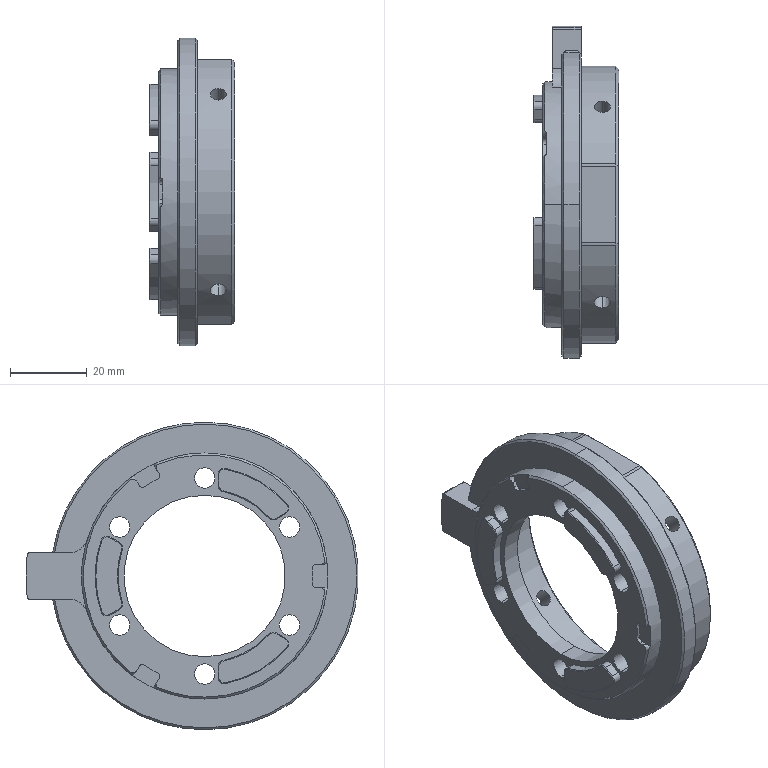NC program | NX | posted with a generic post | part box 22.3 x 86.5 x 80 mm
Lines 26 to 918 of 5076:
(ADAPTIVE_MILLING , TOOL : D10)
N50 T15 M6
N52 G54
N54 G17 G0 G90 X-4.653 Y56.531 S9500 M3
N56 G43 Z30. H15
N58 Z-6.65
N60 G94 G1 Z-9.65 F1000.
N62 X-3.84 Y54.685 F3000.
N64 G3 X-3.278 Y54.149 R1.037
N66 X0.063 Y53.446 R11.74
N68 G2 X10.957 Y51.983 R92.322
N70 X21.093 Y-48.726 R53.11
N72 X10.608 Y-52.015 R70.332
N74 X-18.884 Y49.643 R53.097
N76 X-6.289 Y52.703 R48.18
N78 X0.697 Y52.342 R58.37
N80 X16.022 Y49.494 R65.497
N82 X21.686 Y-47.254 R51.997
N84 X6.969 Y-51.539 R57.357
N86 X-8.626 Y51.279 R52.004
N88 X-0.017 Y51.329 R42.561
N90 X17.335 Y47.887 R62.906
N92 X21.905 Y-45.936 R50.899
N94 X2.392 Y-50.859 R52.826
N96 X-10.178 Y49.875 R50.908
N98 X-0.21 Y50.264 R42.519
N100 X18.185 Y46.397 R60.421
N102 X22.205 Y-44.565 R49.801
N104 X-9.796 Y-48.853 R50.201
N106 X-11.56 Y48.443 R49.811
N108 X0.13 Y49.146 R42.043
N110 X21.213 Y43.868 R55.715
N112 X22.461 Y-43.198 R48.692
N114 X-32.276 Y-36.499 R48.73
N116 X-12.273 Y47.121 R48.677
N118 X0.894 Y48.004 R42.902
N120 X24.046 Y41.104 R52.716
N122 X-47.352 Y5.075 R-47.611
N124 X-12.915 Y45.793 R47.427
N126 X1.477 Y46.867 R43.257
N128 X25.746 Y38.738 R50.676
N130 X7.524 Y-45.874 R46.505
N132 X-14.308 Y44.224 R46.481
N134 X1.271 Y45.786 R42.061
N136 X25.805 Y37.358 R49.355
N138 X-30.481 Y33.648 R-45.391
N140 X-11.505 Y43.805 R43.273
N142 X5.636 Y44.174 R45.023
N144 X31.172 Y31.456 R46.358
N146 X-43.184 Y-9.848 R-44.283
N148 G1 X-43.338 Y-9.304
N150 X-43.35 Y-9.254
N152 X-44.049 Y-5.391
N154 X-44.056 Y-5.34
N156 X-44.379 Y-1.424
N158 X-44.381 Y-1.386
N160 X-44.325 Y2.549
N162 X-44.321 Y2.601
N164 G2 X-43.557 Y8.273 R53.663
N166 X-15.414 Y41.482 R44.351
N168 X1.831 Y43.53 R40.876
N170 X27.351 Y33.407 R46.224
N172 X-28.134 Y-32.742 R-43.172
N174 G1 X-28.675 Y-32.358
N176 X-28.715 Y-32.327
N178 X-31.68 Y-29.753
N180 X-31.717 Y-29.718
N182 X-34.419 Y-26.87
N184 X-34.453 Y-26.831
N186 X-36.868 Y-23.736
N188 X-36.897 Y-23.694
N190 X-39.002 Y-20.38
N192 X-39.028 Y-20.335
N194 X-40.803 Y-16.834
N196 X-40.824 Y-16.787
N198 X-42.253 Y-13.13
N200 X-42.269 Y-13.082
N202 X-43.188 Y-9.834
N204 X-43.35 Y-9.254
N206 X-44.056 Y-5.34
N208 X-44.381 Y-1.386
N210 X-44.321 Y2.601
N212 X-43.878 Y6.553
N214 X-43.069 Y10.395
N216 X-43.056 Y10.444
N218 X-41.88 Y14.19
N220 X-41.862 Y14.238
N222 X-40.329 Y17.852
N224 X-40.307 Y17.899
N226 X-38.433 Y21.348
N228 X-38.406 Y21.392
N230 X-36.207 Y24.645
N232 X-36.177 Y24.686
N234 X-33.674 Y27.711
N236 X-33.64 Y27.749
N238 G2 X-22.244 Y37.008 R56.807
N240 X0.983 Y42.477 R39.115
N242 X27.626 Y31.711 R44.927
N244 X-14.28 Y-39.56 R42.064
N246 G1 X-14.359 Y-39.548
N248 X-15.489 Y-39.287
N250 X-15.55 Y-39.269
N252 G2 X-22.305 Y-36.473 R47.797
N254 X-28.225 Y-32.678 R45.06
N256 G3 X-29.238 Y-32.592 R1.011
N258 G1 X-29.749 Y-32.939 Z-9.619
N260 X-30.243 Y-33.309 Z-9.588
N262 X-30.859 Y-33.762 Z-9.55
N264 X-31.349 Y-34.104
N266 G2 X-32.571 Y-33.843 R1.007
N268 G1 X-35.342 Y-30.459
N270 X-38.093 Y-27.059
N272 G2 X-41.623 Y-21.92 R53.328
N274 X-44.301 Y-16.294 R39.22
N276 X-46.227 Y-10.042 R44.417
N278 X-47.09 Y-5.068 R37.184
N280 G1 X-47.188 Y-3.575
N282 X-47.33 Y0.483
N284 G2 X-46.805 Y6.985 R35.819
N286 X-45.43 Y13.064 R46.25
N288 X-43.008 Y19.138 R42.842
N290 X-39.119 Y25.665 R43.353
N292 X-36.629 Y28.956 R54.71
N294 G1 X-35.319 Y30.552
N296 G2 X-34.345 Y30.897 R1.011
N298 G1 X-34.104 Y30.848
N300 X-32.145 Y30.447 Z-9.65
N302 X-31.506 Y30.327
N304 G3 X-30.819 Y30.552 R1.03
N306 G1 X-27.782 Y33.04
N308 X-27.741 Y33.071
N310 X-24.476 Y35.255
N312 X-24.436 Y35.279
N314 G2 X23.116 Y33.792 R44.536
N316 X-10.193 Y-39.65 R40.949
N318 X-14.28 Y-39.56 R39.491
N320 G3 X-15.024 Y-39.814 R1.026
N322 G1 X-15.356 Y-40.113
N324 X-16.842 Y-41.451 Z-9.55
N326 X-17.082 Y-41.665
N328 X-17.354 Y-41.835
N330 G2 X-18.177 Y-41.81 R1.025
N332 G1 X-23.036 Y-39.422
N334 G2 X-28.56 Y-36.11 R54.922
N336 X-32.749 Y-32.961 R38.545
N338 G1 X-33.565 Y-32.19
N340 X-34.348 Y-31.386
N342 X-35.707 Y-29.91
N344 X-37.027 Y-28.399
N346 G2 X-40.835 Y-23.031 R47.098
N348 X-44.729 Y-14.96 R40.767
N350 X-46.551 Y-8.399 R42.555
N352 X-47.46 Y-0.28 R64.723
N354 X-47.088 Y5.656 R31.632
N356 X-45.028 Y14.131 R47.314
N358 X-39.734 Y24.685 R41.336
N360 X-32.675 Y32.889 R48.607
N362 X-27.382 Y36.895 R35.549
N364 X-22.086 Y40.046 R101.
N366 G1 X-19.387 Y41.536
N368 G2 X-18.189 Y41.36 R1.007
N370 G1 X-17.939 Y41.105
N372 X-16.541 Y39.675 Z-9.65
N374 G3 X-15.49 Y39.286 R1.068
N376 G2 X-12.071 Y39.663 R11.505
N378 X-5.099 Y40.283 R788.852
N380 X5.834 Y39.65 R46.86
N382 X9.041 Y39.268 R10.135
N384 X17.719 Y35.709 R71.914
N386 X32.673 Y-22.721 R39.917
N388 X15.112 Y-36.784 R39.741
N390 G1 X12.628 Y-37.96
N392 X12.582 Y-37.979
N394 X9.041 Y-39.268
N396 X8.979 Y-39.287
N398 G2 X6.186 Y-39.662 R10.36
N400 X-3.18 Y-39.688 R68.393
N402 G1 X-3.554 Y-39.653
N404 X-3.587 Y-39.65
N406 X-10.212
N408 G3 X-11.31 Y-40.752 R1.1
N410 X-10.212 Y-41.85 R1.1
N412 G1 X6.561
N414 G3 X7.659 Y-40.748 R1.1
N416 X6.561 Y-39.65 R1.1
N418 G1 X-3.689
N420 G3 X-4.522 Y-40.098 R1.014
N422 G1 X-4.775 Y-40.478
N424 X-5.879 Y-42.146 Z-9.55
N426 X-6.049 Y-42.401
N428 X-6.26 Y-42.624
N430 G2 X-6.871 Y-42.832 R1.041
N432 G1 X-9.403 Y-42.835
N434 X-11.935 Y-42.819
N436 G2 X-17.906 Y-41.586 R19.072
N438 X-29.335 Y-35.547 R42.918
N440 X-33.433 Y-32.201 R48.256
N442 X-35.907 Y-29.643 R36.08
N444 G1 X-38.152 Y-27.046
N446 G2 X-41.775 Y-21.604 R35.141
N448 X-44.145 Y-16.522 R38.315
N450 X-46.489 Y-8.981 R53.416
N452 G1 X-46.942 Y-7.011
N454 X-47.348 Y-5.031
N456 G2 X-47.605 Y-0.784 R20.073
N458 G1 X-47.506 Y1.296
N460 X-47.392 Y3.376
N462 G2 X-46.479 Y9.113 R37.336
N464 X-42.841 Y19.444 R45.999
N466 X-36.22 Y29.286 R48.06
N468 X-28.961 Y35.853 R44.574
N470 X-22.883 Y39.429 R43.932
N472 X-15.628 Y42.832 R163.757
N474 X-14.306 Y42.333 R1.005
N476 G1 X-14.191 Y42.079
N478 X-13.366 Y40.258 Z-9.65
N480 G3 X-12.446 Y39.65 R1.011
N482 G1 X5.929
N484 G2 X7.849 Y39.548 R15.168
N486 G1 X9.041 Y39.268
N488 X12.692 Y37.933
N490 X16.162 Y36.28
N492 X16.206 Y36.256
N494 X19.505 Y34.282
N496 X19.546 Y34.254
N498 X22.643 Y31.977
N500 X22.683 Y31.945
N502 G2 X32.223 Y21.398 R51.83
N504 X28.494 Y-26.13 R38.687
N506 G1 X27.965 Y-26.806
N508 X27.933 Y-26.843
N510 X25.341 Y-29.589
N512 X25.305 Y-29.624
N514 X22.469 Y-32.117
N516 X22.43 Y-32.148
N518 X19.375 Y-34.368
N520 X19.333 Y-34.395
N522 X16.085 Y-36.321
N524 X16.041 Y-36.344
N526 X15.025 Y-36.825
N528 G3 X15.474 Y-38.729 R1.
N530 G1 X16.462 Y-38.579 Z-9.6
N532 X17.448 Y-38.411 Z-9.55
N534 X18.278 Y-38.277
N536 X19.105 Y-38.123
N538 X19.371 Y-37.99
N540 X22.769 Y-35.585
N542 G3 X29.728 Y-29.349 R46.818
N544 G1 X30.412 Y-28.566
N546 X31.083 Y-27.772
N548 X33.246 Y-25.105
N550 G3 X36.758 Y-19.588 R37.102
N552 X38.514 Y-15.936 R42.392
N554 X41.433 Y-4.041 R44.192
N556 G1 X41.547 Y-2.549
N558 X41.615 Y-1.054
N560 X41.661 Y0.773
N562 X41.654 Y2.601
N564 G3 X41.07 Y7.638 R32.422
N566 X39.399 Y13.635 R35.228
N568 X35.669 Y21.665 R55.912
N570 X34.01 Y24.156 R27.546
N572 G1 X30.171 Y29.258
N574 X29.988 Y29.44
N576 X29.768 Y29.575
N578 X28.156 Y30.271
N580 X26.678 Y30.9 Z-9.63
N582 X26.484 Y30.931 Z-9.64
N584 X26.288 Z-9.65
N586 G3 X25.671 Y29.258 R1.002
N588 G1 X28.199 Y26.53
N590 X28.232 Y26.492
N592 X30.566 Y23.438
N594 X30.595 Y23.397
N596 X32.631 Y20.136
N598 X32.655 Y20.092
N600 X34.374 Y16.653
N602 X34.394 Y16.607
N604 X35.779 Y13.022
N606 X35.795 Y12.974
N608 X36.835 Y9.273
N610 X36.847 Y9.224
N612 X37.533 Y5.442
N614 X37.539 Y5.392
N616 X37.865 Y1.559
N618 X37.866 Y1.518
N620 X37.828 Y-2.333
N622 X37.825 Y-2.383
N624 X37.423 Y-6.206
N626 X37.416 Y-6.255
N628 X36.671 Y-9.958
N630 X36.659 Y-10.005
N632 X35.574 Y-13.623
N634 X35.557 Y-13.669
N636 X34.141 Y-17.17
N638 X34.12 Y-17.215
N640 X32.384 Y-20.569
N642 X32.36 Y-20.612
N644 X30.32 Y-23.79
N646 X30.291 Y-23.83
N648 X28.443 Y-26.194
N650 G3 X28.462 Y-27.461 R1.017
N652 G1 X29.548 Y-28.771
N654 Z-6.65
N656 G0 Z30.
N658 X0.053 Y2.944
N660 Z3.
N662 G3 X0.053 Y2.944 Z2.506 I-3.312 J-3.046 F1000.
N664 X0.053 Y2.944 Z2.013 I-3.312 J-3.046
N666 X0.053 Y2.944 Z1.519 I-3.312 J-3.046
N668 X0.053 Y2.944 Z1.026 I-3.312 J-3.046
N670 X0.053 Y2.944 Z0.532 I-3.312 J-3.046
N672 X0.053 Y2.944 Z0.039 I-3.312 J-3.046
N674 X0.053 Y2.944 Z-0.455 I-3.312 J-3.046
N676 X0.053 Y2.944 Z-0.948 I-3.312 J-3.046
N678 X0.053 Y2.944 Z-1.442 I-3.312 J-3.046
N680 X0.053 Y2.944 Z-1.935 I-3.312 J-3.046
N682 X0.053 Y2.944 Z-2.429 I-3.312 J-3.046
N684 X0.053 Y2.944 Z-2.922 I-3.312 J-3.046
N686 X0.053 Y2.944 Z-3.416 I-3.312 J-3.046
N688 X0.053 Y2.944 Z-3.909 I-3.312 J-3.046
N690 X0.053 Y2.944 Z-4.403 I-3.312 J-3.046
N692 X0.053 Y2.944 Z-4.896 I-3.312 J-3.046
N694 X0.053 Y2.944 Z-5.39 I-3.312 J-3.046
N696 X0.053 Y2.944 Z-5.884 I-3.312 J-3.046
N698 X0.053 Y2.944 Z-6.377 I-3.312 J-3.046
N700 X0.053 Y2.944 Z-6.871 I-3.312 J-3.046
N702 X0.053 Y2.944 Z-7.364 I-3.312 J-3.046
N704 X0.053 Y2.944 Z-7.858 I-3.312 J-3.046
N706 X0.053 Y2.944 Z-8.351 I-3.312 J-3.046
N708 X0.053 Y2.944 Z-8.845 I-3.312 J-3.046
N710 X0.053 Y2.944 Z-9.338 I-3.312 J-3.046
N712 X-3.259 Y-4.603 Z-9.65 R-4.5
N714 X-5.865 Y-3.781 R-4.501 F3000.
N716 X1.609 Y0.889 R4.669
N718 X-6.732 Y-3.688 R-4.977
N720 X1.835 Y1.86 R5.197
N722 X-7.337 Y-3.783 R-5.474
N724 X2.339 Y1.985 R5.712
N726 X-8.13 Y-3.624 R-5.991
N728 X2.709 Y2.514 R6.254
N730 X-8.698 Y-3.77 R-6.536
N732 X3.191 Y2.798 R6.809
N734 X-9.24 Y-3.976 R-7.097
N736 X3.814 Y2.819 R7.382
N738 X-9.954 Y-3.925 R-7.68
N740 X4.254 Y3.298 R7.975
N742 X-6.709 Y7.397 R8.276
N744 X-10.803 Y-3.578 R8.276
N746 X4.988 Y3.144 R8.583
N748 X-11.438 Y-3.683 R-8.895
N750 X5.93 Y2.261 R9.205
N752 X-12.334 Y-3.108 R-9.523
N754 X6.323 Y3.189 R-9.846
N756 X-13.025 Y-3.071 R10.17
N758 X7.293 Y2.129 R10.496
N760 X-13.978 Y-1.859 R10.824
N762 X7.973 Y2.133 R-11.158
N764 X-14.681 Y-1.734 R11.495
N766 X8.777 Y1.413 R11.835
N768 X-15.416 Y-1.373 R12.177
N770 X9.55 Y0.428 R12.521
N772 X-16.176 Y-0.278 R12.868
N774 X10.234 Y-0.81 R13.215
N776 X-16.778 Y1.579 R13.566
N778 X10.695 Y-2.8 R13.919
N780 X-16.152 Y6.155 R14.267
N782 X6.568 Y-11.201 R14.599
N784 X-4.293 Y14.898 R14.9
N786 X-12.264 Y-12.37 R15.156
N788 X10.634 Y7.29 R15.458
N790 X-18.688 Y-3.731 R15.797
N792 X13.17 Y0.666 R16.149
N794 X-19.74 Y1.58 R16.506
N796 X12.171 Y-7.529 R16.856
N798 X-12.082 Y14.761 R17.185
N800 X-4.935 Y-17.612 R17.476
N802 X6.808 Y14.833 R17.768
N804 X-19.741 Y-7.704 R18.095
N806 X15.253 Y2.805 R18.443
N808 X-22.054 Y1.453 R18.8
N810 X9.84 Y-14.327 R19.131
N812 X-2.728 Y19.458 R19.411
N814 X-14.168 Y-16.615 R19.699
N816 X11.651 Y13.715 R20.049
N818 X-23.283 Y-4.298 R20.408
N820 X15.361 Y-9.754 R20.734
N822 X-6.801 Y20.738 R21.013
N824 X-8.398 Y-20.911 R21.301
N826 X7.86 Y18.783 R21.658
N828 X-23.028 Y-9.945 R22.019
N830 X19.281 Y2.209 R22.373
N832 X-24.736 Y7.486 R22.714
N834 X3.68 Y-22.196 R23.001
N836 X4.205 Y22.202 R23.297
N838 X-19.564 Y-17.369 R23.649
N840 X14.413 Y-16.478 R24.034
N842 X13.422 Y17.593 R24.034
N844 X-26.964 Y-6.202 R24.417
N846 X16.734 Y-14.996 R24.734
N848 X-4.465 Y25.019 R24.991
N850 X-6.806 Y-25.334 R25.322
N852 X15.378 Y-17.808 R25.62
N854 X21.372 Y-7.798 R25.452
N856 X22.55 Y1.289 R26.802
N858 X21.446 Y7.608 R28.715
N860 X20.209 Y10.843 R132.37
N862 G1 X18.781 Y13.482
N864 X18.719 Y13.59
N866 X18.656 Y13.698
N868 X18.576 Y13.832
N870 G3 X12.82 Y20.239 R27.567
N872 X5.21 Y24.419 R27.805
N874 X-6.101 Y25.69 R26.945
N876 X-16.522 Y22.182 R26.901
N878 X-21.379 Y18.427 R29.922
N880 X-25.212 Y13.636 R29.9
N882 X-27.807 Y8.076 R29.9
N884 X-29.019 Y2.061 R29.9
N886 G1 X-29.086 Y-0.91
N888 X-29.081 Y-1.012
N890 G3 X-28.115 Y-7.071 R29.9
N892 X-25.748 Y-12.732 R29.9
N894 X-22.113 Y-17.675 R29.9
N896 X-17.416 Y-21.622 R29.919
N898 X-9.338 Y-25.121 R27.839
N900 X-3.243 Y-25.849 R29.463
N902 X5.338 Y-24.376 R27.651
N904 X12.913 Y-20.166 R27.811
N906 X16.998 Y-16.058 R29.766
N908 G1 X18.607 Y-13.789
N910 X18.67 Y-13.688
N912 X20.024 Y-11.234
N914 X20.059 Y-11.165
N916 X20.387 Y-10.452
N918 X20.418 Y-10.377
N920 X21.448 Y-7.604
N922 X21.484 Y-7.484
N924 X22.173 Y-4.631
N926 X22.195 Y-4.507
N928 X22.542 Y-1.593
N930 X22.55 Y-1.467
N932 Y1.467
N934 X22.542 Y1.593
N936 X22.528 Y1.717
N938 X21.528 Y7.304
N940 X21.484 Y7.484
N942 X21.448 Y7.604
N944 X20.417 Y10.381
N946 X20.39 Y10.448
N948 X20.338 Y10.562
N950 X18.781 Y13.482
N952 X18.674 Y13.68
N954 X18.607 Y13.788
N956 X18.534 Y13.89
N958 X16.929 Y16.145
N960 X15.08 Y18.217
N962 X14.996 Y18.302
N964 X12.927 Y20.154
N966 X12.834 Y20.229
N968 X10.57 Y21.838
N970 X10.47 Y21.902
N972 X8.04 Y23.248
N974 X7.933 Y23.3
N976 X5.368 Y24.366
N978 X5.256 Y24.405
N980 X2.587 Y25.178
N982 X2.471 Y25.204
N984 X-0.266 Y25.673
N986 X-0.385 Y25.687
N988 X-0.509 Y25.694
N990 X-3.276 Y25.847
N992 X-6.101 Y25.69
N994 G3 X-6.938 Y24.552 R1.015
N996 G1 X-6.727 Y23.051
N998 Z-6.65
N1000 G0 Z30.
N1002 X-4.681 Y56.558
N1004 Z-11.65
N1006 G1 Z-14.65 F1000.
N1008 X-4.221 Y55.549 F3000.
N1010 X-3.742 Y54.549
N1012 G3 X-3.306 Y54.177 R1.063
N1014 X0.027 Y53.447 R10.851
N1016 G2 X11.656 Y51.83 R87.753
N1018 X19.86 Y-49.24 R53.106
N1020 X9.665 Y-52.196 R71.246
N1022 X-46.174 Y26.253 R53.072
N1024 X-6.458 Y52.701 R52.902
N1026 X-0.095 Y52.414 R48.132
N1028 X13.946 Y50.125 R73.166
N1030 X20.702 Y-47.695 R52.006
N1032 X5.029 Y-51.768 R56.719
N1034 X-8.428 Y51.31 R52.004
N1036 X-0.192 Y51.344 R42.16
N1038 X16.582 Y48.157 R63.918
N1040 X21.161 Y-46.288 R50.907
N1042 X0.071 Y-50.92 R52.509
N1044 X-9.984 Y49.908 R50.906
N1046 X0.236 Y50.23 R42.588
N1048 X19.407 Y45.892 R58.753
N1050 X21.243 Y-45.033 R49.789
N1052 X-11.085 Y-48.575 R50.123
N1054 X-11.126 Y48.535 R49.799
N1056 X0.449 Y49.13 R43.234
N1058 X20.825 Y44.053 R55.907
N1060 X9.833 Y-47.686 R48.707
N1062 X-12.209 Y47.135 R48.689
N1064 X1.459 Y47.966 R43.901
N1066 X22.799 Y41.81 R53.127
N1068 X46.724 Y9.218 R47.692
N1070 G3 X47.077 Y8.662 R3.514
N1072 G2 X48.014 Y6.155 R6.549
N1074 X48.351 Y-2.093 R58.322
N1076 G1 X48.014 Y-6.155
N1078 X48. Y-6.24
N1080 G2 X47.149 Y-8.987 R20.531
N1082 X43.865 Y-18.558 R90.92
N1084 X-36.38 Y-30.727 R47.661
N1086 G1 X-36.621 Y-30.44
N1088 X-36.859 Y-30.15
N1090 X-37.106 Y-29.845
N1092 X-39.374 Y-27.089
N1094 X-39.403 Y-27.051
N1096 X-41.7 Y-23.673
N1098 X-41.725 Y-23.632
N1100 X-43.703 Y-20.059
N1102 X-43.725 Y-20.015
N1104 X-45.368 Y-16.276
N1106 X-45.385 Y-16.231
N1108 X-46.68 Y-12.357
N1110 X-46.693 Y-12.311
N1112 X-47.628 Y-8.335
N1114 X-47.637 Y-8.287
N1116 X-48.204 Y-4.242
N1118 X-48.208 Y-4.194
N1120 X-48.404 Y-0.089
N1122 X-48.225 Y4.014
N1124 X-48.221 Y4.063
N1126 X-47.669 Y8.109
N1128 X-47.661 Y8.157
N1130 X-46.742 Y12.137
N1132 X-46.729 Y12.184
N1134 X-45.45 Y16.062
N1136 X-45.433 Y16.108
N1138 X-43.804 Y19.853
N1140 X-43.783 Y19.897
N1142 X-41.819 Y23.478
N1144 X-41.794 Y23.519
N1146 G2 X-31.315 Y35.877 R58.41
N1148 X-11.29 Y46.179 R45.823
N1150 X4.133 Y46.593 R46.615
N1152 X28.226 Y36.971 R49.601
N1154 X45.246 Y10.885 R47.105
N1156 G3 X46.091 Y9.771 R1.581
N1158 G1 X46.187 Y9.687
N1160 X46.934 Y8.846
N1162 G2 X48.014 Y6.155 R6.351
N1164 G1 X48.352 Y2.049
N1166 X48.351 Y-2.093
N1168 X48. Y-6.24
N1170 X47.697 Y-7.455
N1172 X47.652 Y-7.574
N1174 G2 X46.353 Y-9.832 R40.435
N1176 G3 X44.011 Y-15.489 R79.968
N1178 G2 X33.71 Y-32.046 R50.363
N1180 X-21.517 Y-41.238 R46.63
N1182 G1 X-23.602 Y-40.304
N1184 X-23.646 Y-40.282
N1186 X-27.276 Y-38.228
N1188 X-27.318 Y-38.202
N1190 X-30.671 Y-35.871
N1192 X-30.71 Y-35.842
N1194 X-33.837 Y-33.214
N1196 X-33.872 Y-33.181
N1198 X-36.745 Y-30.279
N1200 X-36.778 Y-30.243
N1202 X-37.175 Y-29.76
N1204 G3 X-38.917 Y-30.639 R1.001
N1206 G1 X-38.699 Y-31.166 Z-14.621
N1208 X-38.454 Y-31.681 Z-14.593
N1210 X-38.094 Y-32.46 Z-14.55
N1212 X-37.344 Y-34.059
N1214 X-37.175 Y-34.26
N1216 X-35.796 Y-35.524
N1218 X-34.383 Y-36.749
N1220 G3 X-27.548 Y-41.473 R58.147
N1222 X-19.897 Y-45.227 R67.301
N1224 X-11.651 Y-48.061 R58.6
N1226 G1 X-8.296 Y-48.922
N1228 G3 X-0.624 Y-49.683 R31.054
N1230 X8.044 Y-48.769 R56.237
N1232 G1 X9.946 Y-48.416
N1234 X11.839 Y-48.016
N1236 G3 X19.967 Y-45.217 R44.748
N1238 X25.485 Y-42.32 R46.569
N1240 X30.203 Y-39.272 R79.669
N1242 X33.745 Y-36.388 R29.88
N1244 G1 X34.33 Y-35.798
N1246 X34.902 Y-35.196
N1248 X36.416 Y-33.534
N1250 X37.898 Y-31.845
N1252 G3 X42.477 Y-25.315 R43.327
N1254 X46.666 Y-17.64 R241.213
N1256 G1 X49.255 Y-12.664
N1258 G3 X49.344 Y-11.986 R1.033
N1260 G1 X48.977 Y-10.333
N1262 X48.839 Y-9.689 Z-14.583
N1264 X48.677 Y-9.052 Z-14.616
N1266 G3 X48.229 Y-8.553 Z-14.65 R1.039
N1268 X47.005 Y-8.767 R1.007
N1270 X44.1 Y-13.08 R13.969
N1272 G2 X39.848 Y-21.851 R118.493
N1274 X-5.722 Y-45.034 R45.642
N1276 G1 X-7.47 Y-44.952
N1278 X-7.52 Y-44.947
N1280 X-11.649 Y-44.362
N1282 X-11.697 Y-44.352
N1284 X-15.754 Y-43.384
N1286 X-15.802 Y-43.37
N1288 X-19.75 Y-42.028
N1290 X-19.796 Y-42.01
N1292 X-21.621 Y-41.192
N1294 G3 X-23.022 Y-41.98 R1.003
N1296 X-22.726 Y-42.847 Z-14.603 R1.147
N1298 G1 X-22.106 Y-43.701 Z-14.55
N1300 X-21.541 Y-44.486
N1302 X-20.96 Y-45.26
N1304 G3 X-20.457 Y-45.538 R1.051
N1306 G1 X-15.673 Y-46.574
N1308 X-10.883 Y-47.576
N1310 X-9.424 Y-47.861
N1312 X-7.962 Y-48.13
N1314 G3 X-2.645 Y-48.483 R29.412
N1316 G1 X1.728 Y-48.355
N1318 G3 X9.151 Y-47.451 R56.509
N1320 X19.263 Y-44.358 R41.96
N1322 X24.782 Y-41.466 R44.858
N1324 X31.657 Y-36.687 R60.043
N1326 X35.461 Y-32.949 R31.966
N1328 X42.678 Y-22.8 R58.296
N1330 G1 X45.053 Y-18.368
N1332 X47.402 Y-13.922
N1334 X47.461 Y-13.685
N1336 X47.702 Y-11.701
N1338 X47.787 Y-11.046 Z-14.583
N1340 X47.848 Y-10.388 Z-14.616
N1342 G3 X47.596 Y-9.772 Z-14.65 R1.039
N1344 X46.187 Y-9.687 R1.005
N1346 X43.48 Y-12.744 R8.296
N1348 X40.002 Y-19.388 R218.961
N1350 G2 X26.545 Y-35.441 R47.236
N1352 X10.133 Y-43.082 R44.95
N1354 G1 X9.206 Y-43.395
N1356 X9.159 Y-43.409
N1358 X5.113 Y-44.367
N1360 X5.065 Y-44.376
N1362 X0.947 Y-44.953
N1364 X0.898 Y-44.957
N1366 X-3.279 Y-45.15
N1368 X-5.789 Y-45.031
N1370 G3 X-6.383 Y-46.867 R1.001
N1372 G1 X-6.013 Y-47.036 Z-14.63
N1374 X-5.63 Y-47.174 Z-14.609
N1376 X-4.519 Y-47.587 Z-14.55
N1378 X-2.875 Y-48.19
N1380 X-2.607 Y-48.213
N1382 X-0.74 Y-48.125
N1384 X1.124 Y-47.983
N1386 G3 X10.299 Y-46.184 R63.114
N1388 X15.675 Y-44.551 R76.492
N1390 X22.862 Y-41.294 R47.031
N1392 X31.334 Y-35.317 R45.135
N1394 X35.179 Y-31.526 R61.541
N1396 X40.1 Y-25.091 R52.378
N1398 G1 X40.772 Y-24.039
N1400 X46.741 Y-14.472
N1402 X46.838 Y-14.257
N1404 X46.889 Y-14.026
N1406 X47.045 Y-12.167
N1408 X47.105 Y-11.515 Z-14.583
N1410 X47.14 Y-10.861 Z-14.616
N1412 G3 X46.856 Y-10.247 Z-14.65 R1.038
N1414 X45.576 Y-10.126 R1.007
N1416 X44.053 Y-11.181 R14.835
N1418 X41.169 Y-15.243 R17.512
N1420 G2 X35.721 Y-24.358 R99.276
N1422 X24.897 Y-35.253 R44.428
N1424 G1 X24.157 Y-35.875
N1426 X24.118 Y-35.905
N1428 X20.699 Y-38.27
N1430 X20.657 Y-38.296
N1432 X17.033 Y-40.334
N1434 X16.989 Y-40.356
N1436 X13.191 Y-42.047
N1438 X13.145 Y-42.065
N1440 X10.066 Y-43.105
N1442 G3 X9.669 Y-44.749 R1.002
N1444 X10.44 Y-45.069 Z-14.607 R1.172
N1446 G1 X11.574 Y-45.223 Z-14.55
N1448 X13.355 Y-45.465
N1450 G3 X13.963 Y-45.355 R1.044
N1452 G1 X16.531 Y-43.975
N1454 X19.092 Y-42.583
N1456 G3 X28.738 Y-36.074 R76.978
N1458 X39.109 Y-24.53 R47.964
N1460 X44.965 Y-15.028 R255.2
N1462 G1 X45.034 Y-14.886
N1464 X45.831 Y-12.88
N1466 X46.077 Y-12.278 Z-14.583
N1468 X46.298 Y-11.666 Z-14.615
N1470 G3 X46.199 Y-10.989 Z-14.65 R1.038
N1472 X44.965 Y-10.528 R1.005
N1474 X41.991 Y-12.711 R6.003
N1476 X38.575 Y-17.938 R45.009
N1478 G1 X37.799 Y-19.222
N1480 X37.539 Y-19.649
N1482 X37.211 Y-20.181
N1484 X37.145 Y-20.287
N1486 X36.744 Y-20.921
N1488 X36.543 Y-21.237
N1490 X36.498 Y-21.306
N1492 X35.342 Y-23.425
N1494 X35.316 Y-23.467
N1496 X32.994 Y-26.915
N1498 X32.965 Y-26.955
N1500 X30.332 Y-30.172
N1502 X30.299 Y-30.209
N1504 X27.377 Y-33.167
N1506 X27.341 Y-33.201
N1508 X24.852 Y-35.291
N1510 G3 X26.425 Y-36.813 R-1.1
N1512 G1 X39.107 Y-20.664
N1514 X40.342 Y-19.091 Z-14.55
N1516 X44.957 Y-13.215
N1518 X45.296 Y-12.789 Z-14.577
N1520 X45.618 Y-12.35 Z-14.605
N1522 G3 X45.694 Y-11.469 Z-14.65 R1.127
N1524 X44.263 Y-10.794 R1.104
N1526 X42.364 Y-11.677 R6.484
N1528 X39.174 Y-15.373 R14.727
N1530 G2 X37.333 Y-19.775 R59.519
N1532 G1 X36.495 Y-21.311
N1534 G3 X38.382 Y-22.439 R1.1
N1536 G1 X38.83 Y-21.751
N1538 X39.923 Y-20.076 Z-14.55
N1540 X44.255 Y-13.435
N1542 X44.82 Y-12.549 Z-14.603
N1544 G3 X44.822 Y-11.629 Z-14.65 R1.117
N1546 X43.69 Y-10.994 R1.108
N1548 X40.806 Y-12.346 R4.691
N1550 X39.798 Y-13.444 R4.217
N1552 G1 X39.144 Y-15.466
N1554 G3 X41.026 Y-16.52 R1.1
N1556 G1 X44.161 Y-12.862
N1558 G3 X43.193 Y-11.054 R1.101
N1560 X40.319 Y-12.141 R4.655
N1562 X39.772 Y-13.526 R4.427
N1564 X41.581 Y-14.658 R1.101
N1566 G1 X43.265 Y-13.037
N1568 G3 X42.436 Y-11.146 R1.101
N1570 X40.679 Y-11.469 R3.243
N1572 X40.082 Y-12.568 R1.88
N1574 X41.929 Y-13.661 R1.101
N1576 G1 X42.303 Y-13.269
N1578 X42.661 Y-12.862
N1580 G3 X41.747 Y-11.15 R1.102
N1582 X40.274 Y-11.973 R1.304
N1584 X41.207 Y-13.293 R1.013
N1586 G1 X41.872 Y-13.307
N1588 X42.537 Y-13.346
N1590 G2 X41.856 Y-15.224 R-1.01
N1592 G1 Z-11.65
N1594 G0 Z30.
N1596 X-40.676 Y29.433
N1598 Z-11.65
N1600 G1 Z-14.65 F1000.
N1602 G3 X-41.897 Y27.857 R1.01 F3000.
N1604 G1 X-41.396 Y27.309
N1606 X-40.877 Y26.78
N1608 G3 X-39.482 Y26.945 R1.015
N1610 G1 X-36.899 Y30.108
N1612 X-36.866 Y30.145
N1614 X-34.005 Y33.059
N1616 X-33.969 Y33.092
N1618 X-30.853 Y35.732
N1620 X-30.815 Y35.761
N1622 X-27.469 Y38.106
N1624 X-27.43 Y38.131
N1626 G2 X-14.656 Y44.123 R61.728
N1628 X1.907 Y45.727 R42.363
N1630 X25.199 Y37.774 R49.368
N1632 X43.649 Y12.571 R45.794
N1634 G3 X44.409 Y10.866 R6.225
N1636 X45.077 Y10.469 R2.281
N1638 G1 X45.798 Y9.973
N1640 G3 X47.059 Y10.077 R1.007
N1642 X47.343 Y11.074 Z-14.596 R1.106
N1644 G1 X47.256 Y11.988 Z-14.55
N1646 X47.048 Y14.083
N1648 X46.963 Y14.32
N1650 X44.73 Y18.691
N1652 X42.474 Y23.05
N1654 G3 X38.664 Y28.947 R47.013
N1656 X29.308 Y38.657 R51.345
N1658 X23.906 Y42.15 R37.95
N1660 X3.801 Y48.501 R56.019
N1662 X-2.01 Y48.884 R71.979
N1664 X-10.736 Y48.152 R45.534
N1666 X-16.514 Y46.606 R41.879
N1668 G1 X-23.001 Y44.356
N1670 G3 X-23.466 Y44.021 R1.052
N1672 G1 X-24.555 Y42.605
N1674 X-25.024 Y42.004 Z-14.588
N1676 X-25.475 Y41.389 Z-14.626
N1678 X-25.559 Y41.168 Z-14.638
N1680 X-25.595 Y40.935 Z-14.65
N1682 G3 X-24.166 Y40.009 R1.002
N1684 G2 X-14.084 Y43.831 R48.403
N1686 X-3.281 Y45.15 R48.867
N1688 G1 X0.898 Y44.957
N1690 X0.947 Y44.953
N1692 G2 X14.064 Y42.07 R64.136
N1694 X42.11 Y13.813 R44.939
N1696 G3 X43.371 Y11.243 R9.632
N1698 X43.813 Y10.964 R3.092
N1700 G1 X44.865 Y10.566
N1702 G3 X46.089 Y11.008 R1.006
N1704 X46.079 Y12.044 Z-14.596 R1.107
N1706 G1 X45.737 Y12.896 Z-14.55
N1708 X43.958 Y17.393
N1710 G3 X38.944 Y26.707 R43.766
N1712 X26.191 Y39.39 R48.726
N1714 X21.877 Y41.887 R38.489
N1716 X13.888 Y45.428 R84.376
N1718 G1 X8.295 Y47.549
N1720 G3 X7.5 Y47.511 R1.026
N1722 G1 X5.951 Y46.752
N1724 X5.351 Y46.462 Z-14.583
N1726 X4.761 Y46.152 Z-14.617
N1728 G3 X4.383 Y45.618 Z-14.65 R1.04
N1730 X5.113 Y44.367 R1.004
N1732 G1 X9.159 Y43.409
N1734 X9.206 Y43.395
N1736 X13.145 Y42.065
N1738 X13.191 Y42.047
N1740 X16.989 Y40.356
N1742 X17.033 Y40.334
N1744 X20.657 Y38.297
N1746 X20.699 Y38.27
N1748 G2 X28.193 Y32.719 R81.938
N1750 X40.495 Y15.049 R44.225
N1752 G3 X42.179 Y11.709 R15.451
N1754 X43.031 Y11.074 R1.508
N1756 G1 X43.69 Y10.994
N1758 X43.811 Y10.964
N1760 G3 X45.087 Y11.605 R1.106
N1762 X44.885 Y12.781 Z-14.587 R1.123
N1764 G1 X44.43 Y13.366 Z-14.55
N1766 X40.826 Y17.997
N1768 X39.598 Y19.575 Z-14.65
N1770 X25.733 Y37.393
N1772 G3 X24.157 Y35.875 R-1.1
N1774 G1 X27.341 Y33.201
N1776 X27.377 Y33.167
N1778 X30.299 Y30.209
N1780 X30.332 Y30.172
N1782 X32.965 Y26.955
N1784 X32.994 Y26.915
N1786 X35.316 Y23.467
N1788 X35.342 Y23.425
N1790 X37.333 Y19.775
N1792 X37.355 Y19.731
N1794 G3 X40.348 Y13.095 R91.457
N1796 X41.713 Y11.326 R5.935
N1798 X42.436 Y11.146 R1.478
N1800 G1 X43.056 Y11.071
N1802 G3 X44.062 Y12.831 R1.101
N1804 G1 X40.901 Y16.967
N1806 G3 X38.997 Y15.911 R1.1
N1808 X40.189 Y12.439 R34.946
N1810 X41.358 Y11.195 R2.286
N1812 X42.341 Y11.15 R6.116
N1814 X43.034 Y13.104 R1.101
N1816 G1 X41.678 Y14.204
N1818 G3 X39.939 Y13.011 R1.101
N1820 G1 X40.274 Y11.973
N1822 X40.323 Y11.858
N1824 X40.356 Y11.784
N1826 X40.384 Y11.731
N1828 G3 X41.633 Y11.15 R1.243